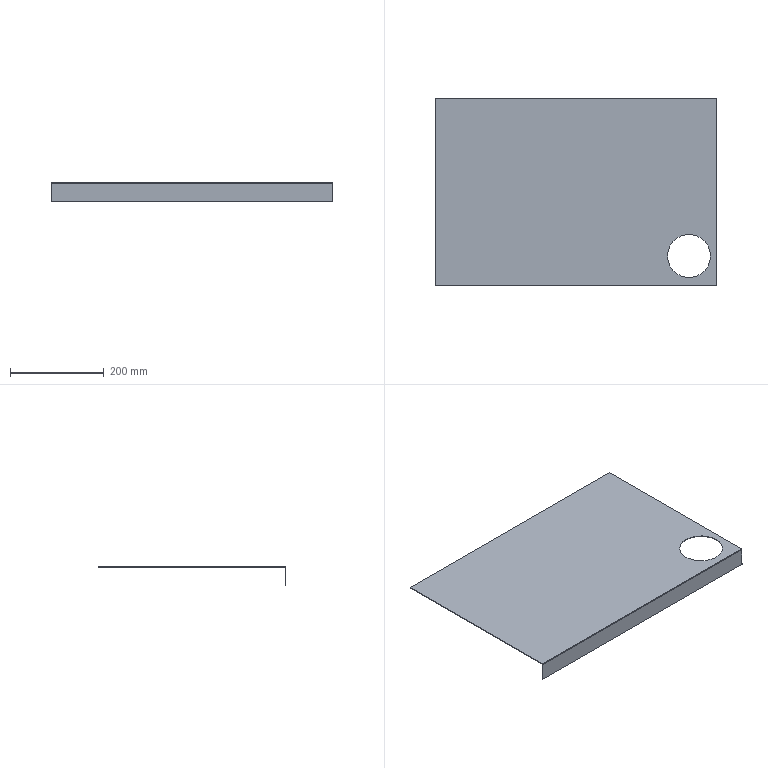Part | SolidWorks | features Cut 1, EdgeFlange 1, FlatPattern 1, SMBaseFlange 1, SheetMetal 1 | 1 solid | 16 faces | box 600 x 400 x 40 mm | volume 384460 mm3 | plane 12 | cylinder 4 | commonest cylinder face diameters 91.493 x2 0.2 x1 3.2 x1
STEP:
#1=CARTESIAN_POINT('',(194.919,-136.309,-1.5));
#2=VERTEX_POINT('',#1);
#3=CARTESIAN_POINT('',(286.412,-136.309,-1.5));
#4=VERTEX_POINT('',#3);
#5=CARTESIAN_POINT('',(240.665,-136.309,-1.5));
#6=DIRECTION('',(0.,0.,1.));
#7=DIRECTION('',(1.,0.,0.));
#8=AXIS2_PLACEMENT_3D('',#5,#6,#7);
#9=CIRCLE('',#8,45.747);
#10=EDGE_CURVE('',#2,#4,#9,.T.);
#11=ORIENTED_EDGE('',*,*,#10,.F.);
#12=CARTESIAN_POINT('',(194.919,-136.309,0.));
#13=VERTEX_POINT('',#12);
#14=CARTESIAN_POINT('',(194.919,-136.309,-20.));
#15=DIRECTION('',(0.,0.,1.));
#16=VECTOR('',#15,1000.);
#17=LINE('',#14,#16);
#18=EDGE_CURVE('',#2,#13,#17,.T.);
#19=ORIENTED_EDGE('',*,*,#18,.T.);
#20=CARTESIAN_POINT('',(286.412,-136.309,0.));
#21=VERTEX_POINT('',#20);
#22=CARTESIAN_POINT('',(240.665,-136.309,0.));
#23=DIRECTION('',(0.,0.,1.));
#24=DIRECTION('',(1.,0.,0.));
#25=AXIS2_PLACEMENT_3D('',#22,#23,#24);
#26=CIRCLE('',#25,45.747);
#27=EDGE_CURVE('',#13,#21,#26,.T.);
#28=ORIENTED_EDGE('',*,*,#27,.T.);
#29=CARTESIAN_POINT('',(286.412,-136.309,-20.));
#30=DIRECTION('',(0.,0.,1.));
#31=VECTOR('',#30,1000.);
#32=LINE('',#29,#31);
#33=EDGE_CURVE('',#4,#21,#32,.T.);
#34=ORIENTED_EDGE('',*,*,#33,.F.);
#35=EDGE_LOOP('',(#11,#19,#28,#34));
#36=FACE_OUTER_BOUND('',#35,.T.);
#37=CARTESIAN_POINT('',(240.665,-136.309,-20.));
#38=DIRECTION('',(0.,0.,1.));
#39=DIRECTION('',(1.,0.,0.));
#40=AXIS2_PLACEMENT_3D('',#37,#38,#39);
#41=CYLINDRICAL_SURFACE('',#40,45.747);
#42=ADVANCED_FACE('',(#36),#41,.F.);
#43=CARTESIAN_POINT('',(-300.,200.,-1.5));
#44=VERTEX_POINT('',#43);
#45=CARTESIAN_POINT('',(-300.,-198.4,-1.5));
#46=VERTEX_POINT('',#45);
#47=CARTESIAN_POINT('',(-300.,200.,-1.5));
#48=DIRECTION('',(0.,-1.,0.));
#49=VECTOR('',#48,1000.);
#50=LINE('',#47,#49);
#51=EDGE_CURVE('',#44,#46,#50,.T.);
#52=ORIENTED_EDGE('',*,*,#51,.T.);
#53=CARTESIAN_POINT('',(-300.,-198.4,0.));
#54=VERTEX_POINT('',#53);
#55=CARTESIAN_POINT('',(-300.,-198.4,-1.5));
#56=DIRECTION('',(0.,0.,1.));
#57=VECTOR('',#56,1000.);
#58=LINE('',#55,#57);
#59=EDGE_CURVE('',#46,#54,#58,.T.);
#60=ORIENTED_EDGE('',*,*,#59,.T.);
#61=CARTESIAN_POINT('',(-300.,200.,0.));
#62=VERTEX_POINT('',#61);
#63=CARTESIAN_POINT('',(-300.,200.,0.));
#64=DIRECTION('',(0.,-1.,0.));
#65=VECTOR('',#64,1000.);
#66=LINE('',#63,#65);
#67=EDGE_CURVE('',#62,#54,#66,.T.);
#68=ORIENTED_EDGE('',*,*,#67,.F.);
#69=CARTESIAN_POINT('',(-300.,200.,-1.5));
#70=DIRECTION('',(0.,0.,1.));
#71=VECTOR('',#70,1000.);
#72=LINE('',#69,#71);
#73=EDGE_CURVE('',#44,#62,#72,.T.);
#74=ORIENTED_EDGE('',*,*,#73,.F.);
#75=EDGE_LOOP('',(#52,#60,#68,#74));
#76=FACE_OUTER_BOUND('',#75,.T.);
#77=CARTESIAN_POINT('',(-300.,200.,-1.5));
#78=DIRECTION('',(-1.,0.,0.));
#79=DIRECTION('',(0.,-1.,0.));
#80=AXIS2_PLACEMENT_3D('',#77,#78,#79);
#81=PLANE('',#80);
#82=ADVANCED_FACE('',(#76),#81,.T.);
#83=CARTESIAN_POINT('',(240.665,-136.309,-1.5));
#84=DIRECTION('',(0.,0.,1.));
#85=DIRECTION('',(1.,0.,0.));
#86=AXIS2_PLACEMENT_3D('',#83,#84,#85);
#87=CIRCLE('',#86,45.747);
#88=EDGE_CURVE('',#4,#2,#87,.T.);
#89=ORIENTED_EDGE('',*,*,#88,.T.);
#90=ORIENTED_EDGE('',*,*,#10,.T.);
#91=EDGE_LOOP('',(#89,#90));
#92=FACE_BOUND('',#91,.T.);
#93=CARTESIAN_POINT('',(300.,-198.4,-1.5));
#94=VERTEX_POINT('',#93);
#95=CARTESIAN_POINT('',(-300.,-198.4,-1.5));
#96=DIRECTION('',(1.,0.,0.));
#97=VECTOR('',#96,1000.);
#98=LINE('',#95,#97);
#99=EDGE_CURVE('',#46,#94,#98,.T.);
#100=ORIENTED_EDGE('',*,*,#99,.F.);
#101=ORIENTED_EDGE('',*,*,#51,.F.);
#102=CARTESIAN_POINT('',(300.,200.,-1.5));
#103=VERTEX_POINT('',#102);
#104=CARTESIAN_POINT('',(-300.,200.,-1.5));
#105=DIRECTION('',(-1.,0.,0.));
#106=VECTOR('',#105,1000.);
#107=LINE('',#104,#106);
#108=EDGE_CURVE('',#103,#44,#107,.T.);
#109=ORIENTED_EDGE('',*,*,#108,.F.);
#110=CARTESIAN_POINT('',(300.,200.,-1.5));
#111=DIRECTION('',(0.,1.,0.));
#112=VECTOR('',#111,1000.);
#113=LINE('',#110,#112);
#114=EDGE_CURVE('',#94,#103,#113,.T.);
#115=ORIENTED_EDGE('',*,*,#114,.F.);
#116=EDGE_LOOP('',(#100,#101,#109,#115));
#117=FACE_OUTER_BOUND('',#116,.T.);
#118=CARTESIAN_POINT('',(0.,0.,-1.5));
#119=DIRECTION('',(0.,0.,1.));
#120=DIRECTION('',(1.,0.,0.));
#121=AXIS2_PLACEMENT_3D('',#118,#119,#120);
#122=PLANE('',#121);
#123=ADVANCED_FACE('',(#92,#117),#122,.F.);
#124=CARTESIAN_POINT('',(240.665,-136.309,0.));
#125=DIRECTION('',(0.,0.,1.));
#126=DIRECTION('',(1.,0.,0.));
#127=AXIS2_PLACEMENT_3D('',#124,#125,#126);
#128=CIRCLE('',#127,45.747);
#129=EDGE_CURVE('',#21,#13,#128,.T.);
#130=ORIENTED_EDGE('',*,*,#129,.F.);
#131=ORIENTED_EDGE('',*,*,#27,.F.);
#132=EDGE_LOOP('',(#130,#131));
#133=FACE_BOUND('',#132,.T.);
#134=ORIENTED_EDGE('',*,*,#67,.T.);
#135=CARTESIAN_POINT('',(300.,-198.4,0.));
#136=VERTEX_POINT('',#135);
#137=CARTESIAN_POINT('',(-300.,-198.4,0.));
#138=DIRECTION('',(1.,0.,0.));
#139=VECTOR('',#138,1000.);
#140=LINE('',#137,#139);
#141=EDGE_CURVE('',#54,#136,#140,.T.);
#142=ORIENTED_EDGE('',*,*,#141,.T.);
#143=CARTESIAN_POINT('',(300.,200.,0.));
#144=VERTEX_POINT('',#143);
#145=CARTESIAN_POINT('',(300.,200.,0.));
#146=DIRECTION('',(0.,1.,0.));
#147=VECTOR('',#146,1000.);
#148=LINE('',#145,#147);
#149=EDGE_CURVE('',#136,#144,#148,.T.);
#150=ORIENTED_EDGE('',*,*,#149,.T.);
#151=CARTESIAN_POINT('',(-300.,200.,0.));
#152=DIRECTION('',(-1.,0.,0.));
#153=VECTOR('',#152,1000.);
#154=LINE('',#151,#153);
#155=EDGE_CURVE('',#144,#62,#154,.T.);
#156=ORIENTED_EDGE('',*,*,#155,.T.);
#157=EDGE_LOOP('',(#134,#142,#150,#156));
#158=FACE_OUTER_BOUND('',#157,.T.);
#159=CARTESIAN_POINT('',(0.,0.,0.));
#160=DIRECTION('',(0.,0.,1.));
#161=DIRECTION('',(1.,0.,0.));
#162=AXIS2_PLACEMENT_3D('',#159,#160,#161);
#163=PLANE('',#162);
#164=ADVANCED_FACE('',(#133,#158),#163,.T.);
#165=CARTESIAN_POINT('',(300.,-198.4,-1.5));
#166=DIRECTION('',(0.,0.,1.));
#167=VECTOR('',#166,1000.);
#168=LINE('',#165,#167);
#169=EDGE_CURVE('',#94,#136,#168,.T.);
#170=ORIENTED_EDGE('',*,*,#169,.F.);
#171=ORIENTED_EDGE('',*,*,#114,.T.);
#172=CARTESIAN_POINT('',(300.,200.,-1.5));
#173=DIRECTION('',(0.,0.,1.));
#174=VECTOR('',#173,1000.);
#175=LINE('',#172,#174);
#176=EDGE_CURVE('',#103,#144,#175,.T.);
#177=ORIENTED_EDGE('',*,*,#176,.T.);
#178=ORIENTED_EDGE('',*,*,#149,.F.);
#179=EDGE_LOOP('',(#170,#171,#177,#178));
#180=FACE_OUTER_BOUND('',#179,.T.);
#181=CARTESIAN_POINT('',(300.,200.,-1.5));
#182=DIRECTION('',(1.,0.,0.));
#183=DIRECTION('',(0.,1.,0.));
#184=AXIS2_PLACEMENT_3D('',#181,#182,#183);
#185=PLANE('',#184);
#186=ADVANCED_FACE('',(#180),#185,.T.);
#187=ORIENTED_EDGE('',*,*,#155,.F.);
#188=ORIENTED_EDGE('',*,*,#176,.F.);
#189=ORIENTED_EDGE('',*,*,#108,.T.);
#190=ORIENTED_EDGE('',*,*,#73,.T.);
#191=EDGE_LOOP('',(#187,#188,#189,#190));
#192=FACE_OUTER_BOUND('',#191,.T.);
#193=CARTESIAN_POINT('',(-300.,200.,-1.5));
#194=DIRECTION('',(0.,1.,0.));
#195=DIRECTION('',(0.,0.,1.));
#196=AXIS2_PLACEMENT_3D('',#193,#194,#195);
#197=PLANE('',#196);
#198=ADVANCED_FACE('',(#192),#197,.T.);
#199=CARTESIAN_POINT('',(300.,-198.5,-1.6));
#200=VERTEX_POINT('',#199);
#201=CARTESIAN_POINT('',(300.,-200.,-1.6));
#202=VERTEX_POINT('',#201);
#203=CARTESIAN_POINT('',(300.,-200.,-1.6));
#204=DIRECTION('',(0.,-1.,0.));
#205=VECTOR('',#204,1000.);
#206=LINE('',#203,#205);
#207=EDGE_CURVE('',#200,#202,#206,.T.);
#208=ORIENTED_EDGE('',*,*,#207,.F.);
#209=CARTESIAN_POINT('',(300.,-198.4,-1.6));
#210=DIRECTION('',(1.,0.,0.));
#211=DIRECTION('',(0.,0.,1.));
#212=AXIS2_PLACEMENT_3D('',#209,#210,#211);
#213=CIRCLE('',#212,0.1);
#214=EDGE_CURVE('',#94,#200,#213,.T.);
#215=ORIENTED_EDGE('',*,*,#214,.F.);
#216=ORIENTED_EDGE('',*,*,#169,.T.);
#217=CARTESIAN_POINT('',(300.,-198.4,-1.6));
#218=DIRECTION('',(1.,0.,0.));
#219=DIRECTION('',(0.,0.,1.));
#220=AXIS2_PLACEMENT_3D('',#217,#218,#219);
#221=CIRCLE('',#220,1.6);
#222=EDGE_CURVE('',#136,#202,#221,.T.);
#223=ORIENTED_EDGE('',*,*,#222,.T.);
#224=EDGE_LOOP('',(#208,#215,#216,#223));
#225=FACE_OUTER_BOUND('',#224,.T.);
#226=CARTESIAN_POINT('',(300.,-198.4,-1.6));
#227=DIRECTION('',(1.,0.,0.));
#228=DIRECTION('',(0.,0.,-1.));
#229=AXIS2_PLACEMENT_3D('',#226,#227,#228);
#230=PLANE('',#229);
#231=ADVANCED_FACE('',(#225),#230,.T.);
#232=CARTESIAN_POINT('',(-300.,-198.5,-1.6));
#233=VERTEX_POINT('',#232);
#234=CARTESIAN_POINT('',(-300.,-198.4,-1.6));
#235=DIRECTION('',(-1.,0.,0.));
#236=DIRECTION('',(0.,0.,1.));
#237=AXIS2_PLACEMENT_3D('',#234,#235,#236);
#238=CIRCLE('',#237,0.1);
#239=EDGE_CURVE('',#233,#46,#238,.T.);
#240=ORIENTED_EDGE('',*,*,#239,.F.);
#241=CARTESIAN_POINT('',(-300.,-200.,-1.6));
#242=VERTEX_POINT('',#241);
#243=CARTESIAN_POINT('',(-300.,-198.5,-1.6));
#244=DIRECTION('',(0.,-1.,0.));
#245=VECTOR('',#244,1000.);
#246=LINE('',#243,#245);
#247=EDGE_CURVE('',#233,#242,#246,.T.);
#248=ORIENTED_EDGE('',*,*,#247,.T.);
#249=CARTESIAN_POINT('',(-300.,-198.4,-1.6));
#250=DIRECTION('',(-1.,0.,0.));
#251=DIRECTION('',(0.,0.,1.));
#252=AXIS2_PLACEMENT_3D('',#249,#250,#251);
#253=CIRCLE('',#252,1.6);
#254=EDGE_CURVE('',#242,#54,#253,.T.);
#255=ORIENTED_EDGE('',*,*,#254,.T.);
#256=ORIENTED_EDGE('',*,*,#59,.F.);
#257=EDGE_LOOP('',(#240,#248,#255,#256));
#258=FACE_OUTER_BOUND('',#257,.T.);
#259=CARTESIAN_POINT('',(-300.,-198.4,-1.6));
#260=DIRECTION('',(1.,0.,0.));
#261=DIRECTION('',(0.,0.,-1.));
#262=AXIS2_PLACEMENT_3D('',#259,#260,#261);
#263=PLANE('',#262);
#264=ADVANCED_FACE('',(#258),#263,.F.);
#265=ORIENTED_EDGE('',*,*,#141,.F.);
#266=ORIENTED_EDGE('',*,*,#254,.F.);
#267=CARTESIAN_POINT('',(0.,-200.,-1.6));
#268=DIRECTION('',(-1.,0.,0.));
#269=VECTOR('',#268,1000.);
#270=LINE('',#267,#269);
#271=EDGE_CURVE('',#202,#242,#270,.T.);
#272=ORIENTED_EDGE('',*,*,#271,.F.);
#273=ORIENTED_EDGE('',*,*,#222,.F.);
#274=EDGE_LOOP('',(#265,#266,#272,#273));
#275=FACE_OUTER_BOUND('',#274,.T.);
#276=CARTESIAN_POINT('',(-300.,-198.4,-1.6));
#277=DIRECTION('',(-1.,0.,0.));
#278=DIRECTION('',(0.,-1.,0.));
#279=AXIS2_PLACEMENT_3D('',#276,#277,#278);
#280=CYLINDRICAL_SURFACE('',#279,1.6);
#281=ADVANCED_FACE('',(#275),#280,.T.);
#282=ORIENTED_EDGE('',*,*,#99,.T.);
#283=ORIENTED_EDGE('',*,*,#214,.T.);
#284=CARTESIAN_POINT('',(300.,-198.5,-1.6));
#285=DIRECTION('',(-1.,0.,0.));
#286=VECTOR('',#285,1000.);
#287=LINE('',#284,#286);
#288=EDGE_CURVE('',#200,#233,#287,.T.);
#289=ORIENTED_EDGE('',*,*,#288,.T.);
#290=ORIENTED_EDGE('',*,*,#239,.T.);
#291=EDGE_LOOP('',(#282,#283,#289,#290));
#292=FACE_OUTER_BOUND('',#291,.T.);
#293=CARTESIAN_POINT('',(-300.,-198.4,-1.6));
#294=DIRECTION('',(-1.,0.,0.));
#295=DIRECTION('',(0.,-1.,0.));
#296=AXIS2_PLACEMENT_3D('',#293,#294,#295);
#297=CYLINDRICAL_SURFACE('',#296,0.1);
#298=ADVANCED_FACE('',(#292),#297,.F.);
#299=CARTESIAN_POINT('',(-300.,-200.,-40.));
#300=VERTEX_POINT('',#299);
#301=CARTESIAN_POINT('',(-300.,-200.,-1.5));
#302=DIRECTION('',(0.,0.,1.));
#303=VECTOR('',#302,1000.);
#304=LINE('',#301,#303);
#305=EDGE_CURVE('',#300,#242,#304,.T.);
#306=ORIENTED_EDGE('',*,*,#305,.T.);
#307=ORIENTED_EDGE('',*,*,#247,.F.);
#308=CARTESIAN_POINT('',(-300.,-198.5,-40.));
#309=VERTEX_POINT('',#308);
#310=CARTESIAN_POINT('',(-300.,-198.5,0.));
#311=DIRECTION('',(0.,0.,1.));
#312=VECTOR('',#311,1000.);
#313=LINE('',#310,#312);
#314=EDGE_CURVE('',#309,#233,#313,.T.);
#315=ORIENTED_EDGE('',*,*,#314,.F.);
#316=CARTESIAN_POINT('',(-300.,-200.,-40.));
#317=DIRECTION('',(0.,1.,0.));
#318=VECTOR('',#317,1000.);
#319=LINE('',#316,#318);
#320=EDGE_CURVE('',#300,#309,#319,.T.);
#321=ORIENTED_EDGE('',*,*,#320,.F.);
#322=EDGE_LOOP('',(#306,#307,#315,#321));
#323=FACE_OUTER_BOUND('',#322,.T.);
#324=CARTESIAN_POINT('',(-300.,-200.,-1.5));
#325=DIRECTION('',(-1.,0.,0.));
#326=DIRECTION('',(0.,0.,1.));
#327=AXIS2_PLACEMENT_3D('',#324,#325,#326);
#328=PLANE('',#327);
#329=ADVANCED_FACE('',(#323),#328,.T.);
#330=CARTESIAN_POINT('',(300.,-198.5,-40.));
#331=VERTEX_POINT('',#330);
#332=CARTESIAN_POINT('',(300.,-198.5,0.));
#333=DIRECTION('',(0.,0.,-1.));
#334=VECTOR('',#333,1000.);
#335=LINE('',#332,#334);
#336=EDGE_CURVE('',#200,#331,#335,.T.);
#337=ORIENTED_EDGE('',*,*,#336,.F.);
#338=ORIENTED_EDGE('',*,*,#207,.T.);
#339=CARTESIAN_POINT('',(300.,-200.,-40.));
#340=VERTEX_POINT('',#339);
#341=CARTESIAN_POINT('',(300.,-200.,-40.));
#342=DIRECTION('',(0.,0.,-1.));
#343=VECTOR('',#342,1000.);
#344=LINE('',#341,#343);
#345=EDGE_CURVE('',#202,#340,#344,.T.);
#346=ORIENTED_EDGE('',*,*,#345,.T.);
#347=CARTESIAN_POINT('',(300.,-200.,-40.));
#348=DIRECTION('',(0.,1.,0.));
#349=VECTOR('',#348,1000.);
#350=LINE('',#347,#349);
#351=EDGE_CURVE('',#340,#331,#350,.T.);
#352=ORIENTED_EDGE('',*,*,#351,.T.);
#353=EDGE_LOOP('',(#337,#338,#346,#352));
#354=FACE_OUTER_BOUND('',#353,.T.);
#355=CARTESIAN_POINT('',(300.,-200.,-40.));
#356=DIRECTION('',(1.,0.,0.));
#357=DIRECTION('',(0.,0.,-1.));
#358=AXIS2_PLACEMENT_3D('',#355,#356,#357);
#359=PLANE('',#358);
#360=ADVANCED_FACE('',(#354),#359,.T.);
#361=ORIENTED_EDGE('',*,*,#345,.F.);
#362=ORIENTED_EDGE('',*,*,#271,.T.);
#363=ORIENTED_EDGE('',*,*,#305,.F.);
#364=CARTESIAN_POINT('',(-300.,-200.,-40.));
#365=DIRECTION('',(-1.,0.,0.));
#366=VECTOR('',#365,1000.);
#367=LINE('',#364,#366);
#368=EDGE_CURVE('',#340,#300,#367,.T.);
#369=ORIENTED_EDGE('',*,*,#368,.F.);
#370=EDGE_LOOP('',(#361,#362,#363,#369));
#371=FACE_OUTER_BOUND('',#370,.T.);
#372=CARTESIAN_POINT('',(0.,-200.,0.));
#373=DIRECTION('',(0.,-1.,0.));
#374=DIRECTION('',(0.,0.,-1.));
#375=AXIS2_PLACEMENT_3D('',#372,#373,#374);
#376=PLANE('',#375);
#377=ADVANCED_FACE('',(#371),#376,.T.);
#378=ORIENTED_EDGE('',*,*,#288,.F.);
#379=ORIENTED_EDGE('',*,*,#336,.T.);
#380=CARTESIAN_POINT('',(0.,-198.5,-40.));
#381=DIRECTION('',(-1.,0.,0.));
#382=VECTOR('',#381,1000.);
#383=LINE('',#380,#382);
#384=EDGE_CURVE('',#331,#309,#383,.T.);
#385=ORIENTED_EDGE('',*,*,#384,.T.);
#386=ORIENTED_EDGE('',*,*,#314,.T.);
#387=EDGE_LOOP('',(#378,#379,#385,#386));
#388=FACE_OUTER_BOUND('',#387,.T.);
#389=CARTESIAN_POINT('',(0.,-198.5,0.));
#390=DIRECTION('',(0.,-1.,0.));
#391=DIRECTION('',(0.,0.,-1.));
#392=AXIS2_PLACEMENT_3D('',#389,#390,#391);
#393=PLANE('',#392);
#394=ADVANCED_FACE('',(#388),#393,.F.);
#395=ORIENTED_EDGE('',*,*,#384,.F.);
#396=ORIENTED_EDGE('',*,*,#351,.F.);
#397=ORIENTED_EDGE('',*,*,#368,.T.);
#398=ORIENTED_EDGE('',*,*,#320,.T.);
#399=EDGE_LOOP('',(#395,#396,#397,#398));
#400=FACE_OUTER_BOUND('',#399,.T.);
#401=CARTESIAN_POINT('',(-300.,-200.,-40.));
#402=DIRECTION('',(0.,0.,-1.));
#403=DIRECTION('',(0.,1.,0.));
#404=AXIS2_PLACEMENT_3D('',#401,#402,#403);
#405=PLANE('',#404);
#406=ADVANCED_FACE('',(#400),#405,.T.);
#407=ORIENTED_EDGE('',*,*,#18,.F.);
#408=ORIENTED_EDGE('',*,*,#88,.F.);
#409=ORIENTED_EDGE('',*,*,#33,.T.);
#410=ORIENTED_EDGE('',*,*,#129,.T.);
#411=EDGE_LOOP('',(#407,#408,#409,#410));
#412=FACE_OUTER_BOUND('',#411,.T.);
#413=CARTESIAN_POINT('',(240.665,-136.309,-20.));
#414=DIRECTION('',(0.,0.,1.));
#415=DIRECTION('',(1.,0.,0.));
#416=AXIS2_PLACEMENT_3D('',#413,#414,#415);
#417=CYLINDRICAL_SURFACE('',#416,45.747);
#418=ADVANCED_FACE('',(#412),#417,.F.);
#419=CLOSED_SHELL('',(#42,#82,#123,#164,#186,#198,#231,#264,#281,#298,#329,#360,#377,#394,#406,#418));
#420=MANIFOLD_SOLID_BREP('',#419);
#421=CARTESIAN_POINT('',(0.,0.,0.));
#422=DIRECTION('',(0.,0.,1.));
#423=DIRECTION('',(1.,0.,0.));
#424=AXIS2_PLACEMENT_3D('',#421,#422,#423);
#425=(LENGTH_UNIT()NAMED_UNIT(*)SI_UNIT(.MILLI.,.METRE.));
#426=UNCERTAINTY_MEASURE_WITH_UNIT(LENGTH_MEASURE(0.00001),#425,'','');
#427=(NAMED_UNIT(*)PLANE_ANGLE_UNIT()SI_UNIT($,.RADIAN.));
#428=(NAMED_UNIT(*)SI_UNIT($,.STERADIAN.)SOLID_ANGLE_UNIT());
#429=(GEOMETRIC_REPRESENTATION_CONTEXT(3)GLOBAL_UNCERTAINTY_ASSIGNED_CONTEXT((#426))GLOBAL_UNIT_ASSIGNED_CONTEXT((#425,#427,#428))REPRESENTATION_CONTEXT('',''));
#430=ADVANCED_BREP_SHAPE_REPRESENTATION('',(#420,#424),#429);